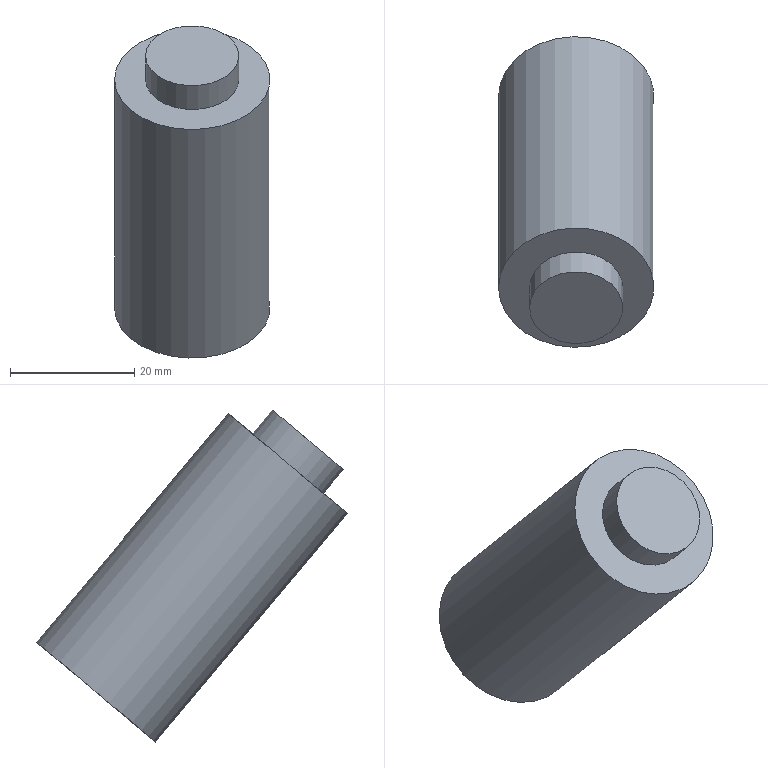Part | NX | features solid 2 | 1 solid | 5 faces | box 25 x 50.005 x 53.456 mm | volume 24446 mm3 | plane 3 | cylinder 2 | commonest cylinder face diameters 15 x1 25 x1
STEP:
#1=CARTESIAN_POINT('',(-527.5,-410.818,-148.253));
#2=VERTEX_POINT('',#1);
#3=CARTESIAN_POINT('',(-515.,-410.818,-148.253));
#4=DIRECTION('',(0.,0.6428,-0.766));
#5=DIRECTION('',(-1.,0.,0.));
#6=AXIS2_PLACEMENT_3D('',#3,#4,#5);
#7=CIRCLE('',#6,12.5);
#8=EDGE_CURVE('',#2,#2,#7,.T.);
#9=ORIENTED_EDGE('',*,*,#8,.F.);
#10=EDGE_LOOP('',(#9));
#11=FACE_BOUND('',#10,.T.);
#12=CARTESIAN_POINT('',(-522.5,-410.818,-148.253));
#13=VERTEX_POINT('',#12);
#14=CARTESIAN_POINT('',(-515.,-410.818,-148.253));
#15=DIRECTION('',(0.,0.6428,-0.766));
#16=DIRECTION('',(-1.,0.,0.));
#17=AXIS2_PLACEMENT_3D('',#14,#15,#16);
#18=CIRCLE('',#17,7.5);
#19=EDGE_CURVE('',#13,#13,#18,.T.);
#20=ORIENTED_EDGE('',*,*,#19,.T.);
#21=EDGE_LOOP('',(#20));
#22=FACE_BOUND('',#21,.T.);
#23=CARTESIAN_POINT('',(-515.,-410.818,-148.253));
#24=DIRECTION('',(0.,-0.6428,0.766));
#25=DIRECTION('',(-1.,0.,0.));
#26=AXIS2_PLACEMENT_3D('',#23,#24,#25);
#27=PLANE('',#26);
#28=ADVANCED_FACE('',(#11,#22),#27,.T.);
#29=ORIENTED_EDGE('',*,*,#8,.T.);
#30=EDGE_LOOP('',(#29));
#31=FACE_BOUND('',#30,.T.);
#32=CARTESIAN_POINT('',(-527.5,-379.964,-185.023));
#33=VERTEX_POINT('',#32);
#34=CARTESIAN_POINT('',(-515.,-379.964,-185.023));
#35=DIRECTION('',(0.,0.6428,-0.766));
#36=DIRECTION('',(-1.,0.,0.));
#37=AXIS2_PLACEMENT_3D('',#34,#35,#36);
#38=CIRCLE('',#37,12.5);
#39=EDGE_CURVE('',#33,#33,#38,.T.);
#40=ORIENTED_EDGE('',*,*,#39,.F.);
#41=EDGE_LOOP('',(#40));
#42=FACE_BOUND('',#41,.T.);
#43=CARTESIAN_POINT('',(-515.,-411.461,-147.487));
#44=DIRECTION('',(0.,0.6428,-0.766));
#45=DIRECTION('',(1.,0.,0.));
#46=AXIS2_PLACEMENT_3D('',#43,#44,#45);
#47=CYLINDRICAL_SURFACE('',#46,12.5);
#48=ADVANCED_FACE('',(#31,#42),#47,.T.);
#49=ORIENTED_EDGE('',*,*,#39,.T.);
#50=EDGE_LOOP('',(#49));
#51=FACE_BOUND('',#50,.T.);
#52=CARTESIAN_POINT('',(-515.,-379.964,-185.023));
#53=DIRECTION('',(0.,-0.6428,0.766));
#54=DIRECTION('',(-1.,0.,0.));
#55=AXIS2_PLACEMENT_3D('',#52,#53,#54);
#56=PLANE('',#55);
#57=ADVANCED_FACE('',(#51),#56,.F.);
#58=CARTESIAN_POINT('',(-522.5,-414.032,-144.423));
#59=VERTEX_POINT('',#58);
#60=CARTESIAN_POINT('',(-515.,-414.032,-144.423));
#61=DIRECTION('',(0.,0.6428,-0.766));
#62=DIRECTION('',(-1.,0.,0.));
#63=AXIS2_PLACEMENT_3D('',#60,#61,#62);
#64=CIRCLE('',#63,7.5);
#65=EDGE_CURVE('',#59,#59,#64,.T.);
#66=ORIENTED_EDGE('',*,*,#65,.T.);
#67=EDGE_LOOP('',(#66));
#68=FACE_BOUND('',#67,.T.);
#69=ORIENTED_EDGE('',*,*,#19,.F.);
#70=EDGE_LOOP('',(#69));
#71=FACE_BOUND('',#70,.T.);
#72=CARTESIAN_POINT('',(-515.,-417.246,-140.593));
#73=DIRECTION('',(0.,0.6428,-0.766));
#74=DIRECTION('',(1.,0.,0.));
#75=AXIS2_PLACEMENT_3D('',#72,#73,#74);
#76=CYLINDRICAL_SURFACE('',#75,7.5);
#77=ADVANCED_FACE('',(#68,#71),#76,.T.);
#78=ORIENTED_EDGE('',*,*,#65,.F.);
#79=EDGE_LOOP('',(#78));
#80=FACE_BOUND('',#79,.T.);
#81=CARTESIAN_POINT('',(-515.,-414.032,-144.423));
#82=DIRECTION('',(0.,-0.6428,0.766));
#83=DIRECTION('',(-1.,0.,0.));
#84=AXIS2_PLACEMENT_3D('',#81,#82,#83);
#85=PLANE('',#84);
#86=ADVANCED_FACE('',(#80),#85,.T.);
#87=CLOSED_SHELL('',(#28,#48,#57,#77,#86));
#88=MANIFOLD_SOLID_BREP('',#87);
#89=(LENGTH_UNIT()NAMED_UNIT(*)SI_UNIT(.MILLI.,.METRE.));
#90=UNCERTAINTY_MEASURE_WITH_UNIT(LENGTH_MEASURE(0.00001),#89,'','');
#91=(NAMED_UNIT(*)PLANE_ANGLE_UNIT()SI_UNIT($,.RADIAN.));
#92=(NAMED_UNIT(*)SI_UNIT($,.STERADIAN.)SOLID_ANGLE_UNIT());
#93=(GEOMETRIC_REPRESENTATION_CONTEXT(3)GLOBAL_UNCERTAINTY_ASSIGNED_CONTEXT((#90))GLOBAL_UNIT_ASSIGNED_CONTEXT((#89,#91,#92))REPRESENTATION_CONTEXT('',''));
#94=ADVANCED_BREP_SHAPE_REPRESENTATION('',(#88),#93);